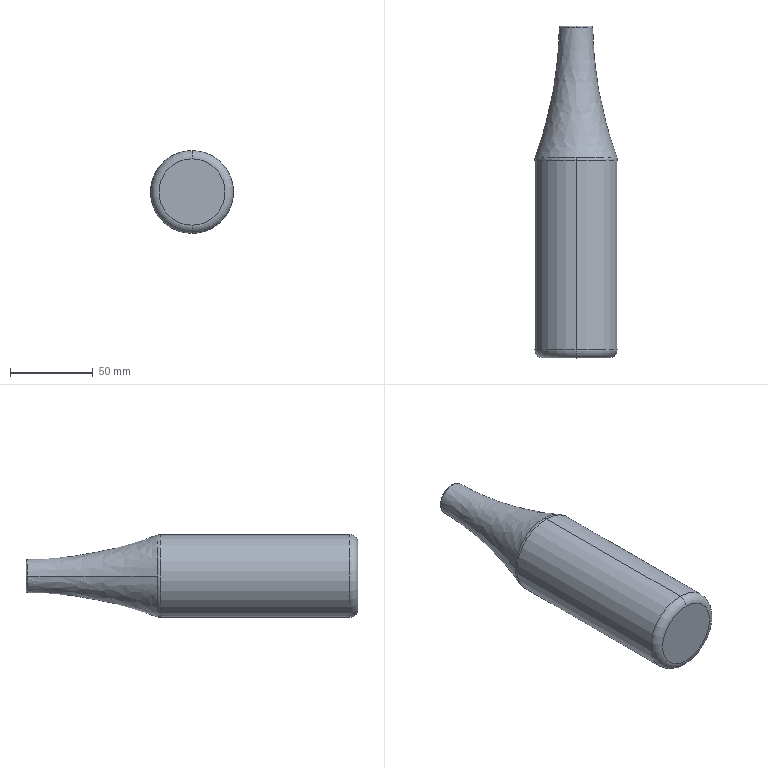Part | SolidWorks | features Fillet 2, Revolution 1, Shell 1 | 1 solid | 21 faces | box 50 x 200 x 50 mm | volume 77937 mm3 | torus 10 | spline 4 | cylinder 4 | plane 3 | commonest cylinder face diameters 44 x2 50 x2
STEP:
#1=CARTESIAN_POINT('',(-93.039,134.747,-7.013));
#2=VERTEX_POINT('',#1);
#3=CARTESIAN_POINT('',(-93.039,134.732,-7.013));
#4=VERTEX_POINT('',#3);
#5=CARTESIAN_POINT('',(-93.039,134.747,-8.013));
#6=DIRECTION('',(1.,0.,0.));
#7=DIRECTION('',(0.,0.,-1.));
#8=AXIS2_PLACEMENT_3D('',#5,#6,#7);
#9=CIRCLE('',#8,1.);
#10=EDGE_CURVE('',#2,#4,#9,.T.);
#11=ORIENTED_EDGE('',*,*,#10,.F.);
#12=CARTESIAN_POINT('',(-93.039,134.747,7.013));
#13=VERTEX_POINT('',#12);
#14=CARTESIAN_POINT('',(-93.039,134.747,0.));
#15=DIRECTION('',(0.,1.,0.));
#16=DIRECTION('',(0.,0.,1.));
#17=AXIS2_PLACEMENT_3D('',#14,#15,#16);
#18=CIRCLE('',#17,7.013);
#19=EDGE_CURVE('',#2,#13,#18,.T.);
#20=ORIENTED_EDGE('',*,*,#19,.T.);
#21=CARTESIAN_POINT('',(-93.039,134.732,7.013));
#22=VERTEX_POINT('',#21);
#23=CARTESIAN_POINT('',(-93.039,134.747,8.013));
#24=DIRECTION('',(-1.,0.,0.));
#25=DIRECTION('',(0.,0.,1.));
#26=AXIS2_PLACEMENT_3D('',#23,#24,#25);
#27=CIRCLE('',#26,1.);
#28=EDGE_CURVE('',#13,#22,#27,.T.);
#29=ORIENTED_EDGE('',*,*,#28,.T.);
#30=CARTESIAN_POINT('',(-100.052,134.732,0.));
#31=VERTEX_POINT('',#30);
#32=CARTESIAN_POINT('',(-93.039,134.732,0.));
#33=DIRECTION('',(0.,1.,0.));
#34=DIRECTION('',(0.,0.,1.));
#35=AXIS2_PLACEMENT_3D('',#32,#33,#34);
#36=CIRCLE('',#35,7.013);
#37=EDGE_CURVE('',#31,#22,#36,.T.);
#38=ORIENTED_EDGE('',*,*,#37,.F.);
#39=CARTESIAN_POINT('',(-93.039,134.732,0.));
#40=DIRECTION('',(0.,1.,0.));
#41=DIRECTION('',(0.,0.,1.));
#42=AXIS2_PLACEMENT_3D('',#39,#40,#41);
#43=CIRCLE('',#42,7.013);
#44=EDGE_CURVE('',#4,#31,#43,.T.);
#45=ORIENTED_EDGE('',*,*,#44,.F.);
#46=EDGE_LOOP('',(#11,#20,#29,#38,#45));
#47=FACE_OUTER_BOUND('',#46,.T.);
#48=CARTESIAN_POINT('',(-93.039,134.747,0.));
#49=DIRECTION('',(0.,1.,0.));
#50=DIRECTION('',(0.,0.,1.));
#51=AXIS2_PLACEMENT_3D('',#48,#49,#50);
#52=TOROIDAL_SURFACE('',#51,8.013,1.);
#53=ADVANCED_FACE('',(#47),#52,.T.);
#54=CARTESIAN_POINT('',(-86.026,134.732,0.));
#55=VERTEX_POINT('',#54);
#56=CARTESIAN_POINT('',(-93.039,134.732,0.));
#57=DIRECTION('',(0.,1.,0.));
#58=DIRECTION('',(0.,0.,1.));
#59=AXIS2_PLACEMENT_3D('',#56,#57,#58);
#60=CIRCLE('',#59,7.013);
#61=EDGE_CURVE('',#22,#55,#60,.T.);
#62=ORIENTED_EDGE('',*,*,#61,.T.);
#63=CARTESIAN_POINT('',(-71.039,55.211,0.));
#64=VERTEX_POINT('',#63);
#65=CARTESIAN_POINT('',(-86.026,134.732,0.));
#66=CARTESIAN_POINT('',(-85.624,107.792,0.));
#67=CARTESIAN_POINT('',(-80.621,81.268,0.));
#68=CARTESIAN_POINT('',(-71.039,55.211,0.));
#69=B_SPLINE_CURVE_WITH_KNOTS('',3,(#65,#66,#67,#68),.UNSPECIFIED.,.F.,.F.,(4,4),(0.01123,0.9355),.UNSPECIFIED.);
#70=EDGE_CURVE('',#55,#64,#69,.T.);
#71=ORIENTED_EDGE('',*,*,#70,.T.);
#72=CARTESIAN_POINT('',(-93.039,55.211,22.));
#73=VERTEX_POINT('',#72);
#74=CARTESIAN_POINT('',(-93.039,55.211,0.));
#75=DIRECTION('',(0.,1.,0.));
#76=DIRECTION('',(0.,0.,1.));
#77=AXIS2_PLACEMENT_3D('',#74,#75,#76);
#78=CIRCLE('',#77,22.);
#79=EDGE_CURVE('',#73,#64,#78,.T.);
#80=ORIENTED_EDGE('',*,*,#79,.F.);
#81=CARTESIAN_POINT('',(-115.039,55.211,0.));
#82=VERTEX_POINT('',#81);
#83=CARTESIAN_POINT('',(-93.039,55.211,0.));
#84=DIRECTION('',(0.,1.,0.));
#85=DIRECTION('',(0.,0.,1.));
#86=AXIS2_PLACEMENT_3D('',#83,#84,#85);
#87=CIRCLE('',#86,22.);
#88=EDGE_CURVE('',#82,#73,#87,.T.);
#89=ORIENTED_EDGE('',*,*,#88,.F.);
#90=CARTESIAN_POINT('',(-100.052,134.732,0.));
#91=CARTESIAN_POINT('',(-100.455,107.792,0.));
#92=CARTESIAN_POINT('',(-105.457,81.268,0.));
#93=CARTESIAN_POINT('',(-115.039,55.211,0.));
#94=B_SPLINE_CURVE_WITH_KNOTS('',3,(#90,#91,#92,#93),.UNSPECIFIED.,.F.,.F.,(4,4),(0.01123,0.9355),.UNSPECIFIED.);
#95=EDGE_CURVE('',#31,#82,#94,.T.);
#96=ORIENTED_EDGE('',*,*,#95,.F.);
#97=ORIENTED_EDGE('',*,*,#37,.T.);
#98=EDGE_LOOP('',(#62,#71,#80,#89,#96,#97));
#99=FACE_OUTER_BOUND('',#98,.T.);
#100=CARTESIAN_POINT('',(-100.052,134.732,0.));
#101=CARTESIAN_POINT('',(-100.052,134.732,14.026));
#102=CARTESIAN_POINT('',(-86.026,134.732,14.026));
#103=CARTESIAN_POINT('',(-86.026,134.732,0.));
#104=CARTESIAN_POINT('',(-100.455,107.792,0.));
#105=CARTESIAN_POINT('',(-100.455,107.792,14.831));
#106=CARTESIAN_POINT('',(-85.624,107.792,14.831));
#107=CARTESIAN_POINT('',(-85.624,107.792,0.));
#108=CARTESIAN_POINT('',(-105.457,81.268,0.));
#109=CARTESIAN_POINT('',(-105.457,81.268,24.836));
#110=CARTESIAN_POINT('',(-80.621,81.268,24.836));
#111=CARTESIAN_POINT('',(-80.621,81.268,0.));
#112=CARTESIAN_POINT('',(-115.039,55.211,0.));
#113=CARTESIAN_POINT('',(-115.039,55.211,44.));
#114=CARTESIAN_POINT('',(-71.039,55.211,44.));
#115=CARTESIAN_POINT('',(-71.039,55.211,0.));
#116=(BOUNDED_SURFACE()B_SPLINE_SURFACE(3,3,((#100,#101,#102,#103),(#104,#105,#106,#107),(#108,#109,#110,#111),(#112,#113,#114,#115)),.UNSPECIFIED.,.F.,.F.,.T.)B_SPLINE_SURFACE_WITH_KNOTS((4,4),(4,4),(0.,1.),(0.,1.),.UNSPECIFIED.)GEOMETRIC_REPRESENTATION_ITEM()RATIONAL_B_SPLINE_SURFACE(((1.,0.3333,0.3333,1.),(1.,0.3333,0.3333,1.),(1.,0.3333,0.3333,1.),(1.,0.3333,0.3333,1.)))REPRESENTATION_ITEM('')SURFACE());
#117=ADVANCED_FACE('',(#99),#116,.F.);
#118=CARTESIAN_POINT('',(-93.039,134.762,-10.013));
#119=VERTEX_POINT('',#118);
#120=CARTESIAN_POINT('',(-83.027,134.762,0.));
#121=VERTEX_POINT('',#120);
#122=CARTESIAN_POINT('',(-93.039,134.762,0.));
#123=DIRECTION('',(0.,-1.,0.));
#124=DIRECTION('',(0.,0.,1.));
#125=AXIS2_PLACEMENT_3D('',#122,#123,#124);
#126=CIRCLE('',#125,10.013);
#127=EDGE_CURVE('',#119,#121,#126,.T.);
#128=ORIENTED_EDGE('',*,*,#127,.T.);
#129=CARTESIAN_POINT('',(-68.344,56.575,0.));
#130=VERTEX_POINT('',#129);
#131=CARTESIAN_POINT('',(-83.027,134.762,0.));
#132=CARTESIAN_POINT('',(-82.431,95.042,0.));
#133=CARTESIAN_POINT('',(-68.344,56.575,0.));
#134=B_SPLINE_CURVE_WITH_KNOTS('',2,(#131,#132,#133),.UNSPECIFIED.,.F.,.F.,(3,3),(0.01141,0.9316),.UNSPECIFIED.);
#135=EDGE_CURVE('',#121,#130,#134,.T.);
#136=ORIENTED_EDGE('',*,*,#135,.T.);
#137=CARTESIAN_POINT('',(-93.039,56.575,-24.695));
#138=VERTEX_POINT('',#137);
#139=CARTESIAN_POINT('',(-93.039,56.575,0.));
#140=DIRECTION('',(0.,1.,0.));
#141=DIRECTION('',(0.,0.,1.));
#142=AXIS2_PLACEMENT_3D('',#139,#140,#141);
#143=CIRCLE('',#142,24.695);
#144=EDGE_CURVE('',#130,#138,#143,.T.);
#145=ORIENTED_EDGE('',*,*,#144,.T.);
#146=CARTESIAN_POINT('',(-117.734,56.575,0.));
#147=VERTEX_POINT('',#146);
#148=CARTESIAN_POINT('',(-93.039,56.575,0.));
#149=DIRECTION('',(0.,1.,0.));
#150=DIRECTION('',(0.,0.,1.));
#151=AXIS2_PLACEMENT_3D('',#148,#149,#150);
#152=CIRCLE('',#151,24.695);
#153=EDGE_CURVE('',#138,#147,#152,.T.);
#154=ORIENTED_EDGE('',*,*,#153,.T.);
#155=CARTESIAN_POINT('',(-103.052,134.762,0.));
#156=VERTEX_POINT('',#155);
#157=CARTESIAN_POINT('',(-103.052,134.762,0.));
#158=CARTESIAN_POINT('',(-103.648,95.042,0.));
#159=CARTESIAN_POINT('',(-117.734,56.575,0.));
#160=B_SPLINE_CURVE_WITH_KNOTS('',2,(#157,#158,#159),.UNSPECIFIED.,.F.,.F.,(3,3),(0.01141,0.9316),.UNSPECIFIED.);
#161=EDGE_CURVE('',#156,#147,#160,.T.);
#162=ORIENTED_EDGE('',*,*,#161,.F.);
#163=CARTESIAN_POINT('',(-93.039,134.762,0.));
#164=DIRECTION('',(0.,-1.,0.));
#165=DIRECTION('',(0.,0.,1.));
#166=AXIS2_PLACEMENT_3D('',#163,#164,#165);
#167=CIRCLE('',#166,10.013);
#168=EDGE_CURVE('',#156,#119,#167,.T.);
#169=ORIENTED_EDGE('',*,*,#168,.T.);
#170=EDGE_LOOP('',(#128,#136,#145,#154,#162,#169));
#171=FACE_OUTER_BOUND('',#170,.T.);
#172=CARTESIAN_POINT('',(-83.027,134.762,0.));
#173=CARTESIAN_POINT('',(-83.027,134.762,-20.025));
#174=CARTESIAN_POINT('',(-103.052,134.762,-20.025));
#175=CARTESIAN_POINT('',(-103.052,134.762,0.));
#176=CARTESIAN_POINT('',(-82.431,95.042,0.));
#177=CARTESIAN_POINT('',(-82.431,95.042,-21.217));
#178=CARTESIAN_POINT('',(-103.648,95.042,-21.217));
#179=CARTESIAN_POINT('',(-103.648,95.042,0.));
#180=CARTESIAN_POINT('',(-68.344,56.575,0.));
#181=CARTESIAN_POINT('',(-68.344,56.575,-49.39));
#182=CARTESIAN_POINT('',(-117.734,56.575,-49.39));
#183=CARTESIAN_POINT('',(-117.734,56.575,0.));
#184=(BOUNDED_SURFACE()B_SPLINE_SURFACE(2,3,((#172,#173,#174,#175),(#176,#177,#178,#179),(#180,#181,#182,#183)),.UNSPECIFIED.,.F.,.F.,.F.)B_SPLINE_SURFACE_WITH_KNOTS((3,3),(4,4),(0.01141,0.9316),(0.,1.),.UNSPECIFIED.)GEOMETRIC_REPRESENTATION_ITEM()RATIONAL_B_SPLINE_SURFACE(((1.,0.3333,0.3333,1.),(1.,0.3333,0.3333,1.),(1.,0.3333,0.3333,1.)))REPRESENTATION_ITEM('')SURFACE());
#185=ADVANCED_FACE('',(#171),#184,.T.);
#186=ORIENTED_EDGE('',*,*,#28,.F.);
#187=CARTESIAN_POINT('',(-93.039,134.747,0.));
#188=DIRECTION('',(0.,1.,0.));
#189=DIRECTION('',(0.,0.,1.));
#190=AXIS2_PLACEMENT_3D('',#187,#188,#189);
#191=CIRCLE('',#190,7.013);
#192=EDGE_CURVE('',#13,#2,#191,.T.);
#193=ORIENTED_EDGE('',*,*,#192,.T.);
#194=ORIENTED_EDGE('',*,*,#10,.T.);
#195=CARTESIAN_POINT('',(-93.039,134.732,0.));
#196=DIRECTION('',(0.,1.,0.));
#197=DIRECTION('',(0.,0.,1.));
#198=AXIS2_PLACEMENT_3D('',#195,#196,#197);
#199=CIRCLE('',#198,7.013);
#200=EDGE_CURVE('',#55,#4,#199,.T.);
#201=ORIENTED_EDGE('',*,*,#200,.F.);
#202=ORIENTED_EDGE('',*,*,#61,.F.);
#203=EDGE_LOOP('',(#186,#193,#194,#201,#202));
#204=FACE_OUTER_BOUND('',#203,.T.);
#205=CARTESIAN_POINT('',(-93.039,134.747,0.));
#206=DIRECTION('',(0.,1.,0.));
#207=DIRECTION('',(0.,0.,1.));
#208=AXIS2_PLACEMENT_3D('',#205,#206,#207);
#209=TOROIDAL_SURFACE('',#208,8.013,1.);
#210=ADVANCED_FACE('',(#204),#209,.T.);
#211=ORIENTED_EDGE('',*,*,#192,.F.);
#212=CARTESIAN_POINT('',(-93.039,135.747,8.013));
#213=VERTEX_POINT('',#212);
#214=CARTESIAN_POINT('',(-93.039,134.747,8.013));
#215=DIRECTION('',(-1.,0.,0.));
#216=DIRECTION('',(0.,0.,1.));
#217=AXIS2_PLACEMENT_3D('',#214,#215,#216);
#218=CIRCLE('',#217,1.);
#219=EDGE_CURVE('',#213,#13,#218,.T.);
#220=ORIENTED_EDGE('',*,*,#219,.F.);
#221=CARTESIAN_POINT('',(-93.039,135.747,-8.013));
#222=VERTEX_POINT('',#221);
#223=CARTESIAN_POINT('',(-93.039,135.747,0.));
#224=DIRECTION('',(0.,-1.,0.));
#225=DIRECTION('',(0.,0.,1.));
#226=AXIS2_PLACEMENT_3D('',#223,#224,#225);
#227=CIRCLE('',#226,8.013);
#228=EDGE_CURVE('',#222,#213,#227,.T.);
#229=ORIENTED_EDGE('',*,*,#228,.F.);
#230=CARTESIAN_POINT('',(-93.039,134.747,-8.013));
#231=DIRECTION('',(1.,0.,0.));
#232=DIRECTION('',(0.,0.,-1.));
#233=AXIS2_PLACEMENT_3D('',#230,#231,#232);
#234=CIRCLE('',#233,1.);
#235=EDGE_CURVE('',#222,#2,#234,.T.);
#236=ORIENTED_EDGE('',*,*,#235,.T.);
#237=EDGE_LOOP('',(#211,#220,#229,#236));
#238=FACE_OUTER_BOUND('',#237,.T.);
#239=CARTESIAN_POINT('',(-93.039,134.747,0.));
#240=DIRECTION('',(0.,1.,0.));
#241=DIRECTION('',(0.,0.,1.));
#242=AXIS2_PLACEMENT_3D('',#239,#240,#241);
#243=TOROIDAL_SURFACE('',#242,8.013,1.);
#244=ADVANCED_FACE('',(#238),#243,.T.);
#245=ORIENTED_EDGE('',*,*,#127,.F.);
#246=CARTESIAN_POINT('',(-93.039,135.747,-9.013));
#247=VERTEX_POINT('',#246);
#248=CARTESIAN_POINT('',(-93.039,134.747,-9.013));
#249=DIRECTION('',(1.,0.,0.));
#250=DIRECTION('',(0.,0.,-1.));
#251=AXIS2_PLACEMENT_3D('',#248,#249,#250);
#252=CIRCLE('',#251,1.);
#253=EDGE_CURVE('',#119,#247,#252,.T.);
#254=ORIENTED_EDGE('',*,*,#253,.T.);
#255=CARTESIAN_POINT('',(-93.039,135.747,9.013));
#256=VERTEX_POINT('',#255);
#257=CARTESIAN_POINT('',(-93.039,135.747,0.));
#258=DIRECTION('',(0.,1.,0.));
#259=DIRECTION('',(0.,0.,1.));
#260=AXIS2_PLACEMENT_3D('',#257,#258,#259);
#261=CIRCLE('',#260,9.013);
#262=EDGE_CURVE('',#256,#247,#261,.T.);
#263=ORIENTED_EDGE('',*,*,#262,.F.);
#264=CARTESIAN_POINT('',(-93.039,134.762,10.013));
#265=VERTEX_POINT('',#264);
#266=CARTESIAN_POINT('',(-93.039,134.747,9.013));
#267=DIRECTION('',(-1.,0.,0.));
#268=DIRECTION('',(0.,0.,1.));
#269=AXIS2_PLACEMENT_3D('',#266,#267,#268);
#270=CIRCLE('',#269,1.);
#271=EDGE_CURVE('',#265,#256,#270,.T.);
#272=ORIENTED_EDGE('',*,*,#271,.F.);
#273=CARTESIAN_POINT('',(-93.039,134.762,0.));
#274=DIRECTION('',(0.,-1.,0.));
#275=DIRECTION('',(0.,0.,1.));
#276=AXIS2_PLACEMENT_3D('',#273,#274,#275);
#277=CIRCLE('',#276,10.013);
#278=EDGE_CURVE('',#121,#265,#277,.T.);
#279=ORIENTED_EDGE('',*,*,#278,.F.);
#280=EDGE_LOOP('',(#245,#254,#263,#272,#279));
#281=FACE_OUTER_BOUND('',#280,.T.);
#282=CARTESIAN_POINT('',(-93.039,134.747,0.));
#283=DIRECTION('',(0.,1.,0.));
#284=DIRECTION('',(0.,0.,1.));
#285=AXIS2_PLACEMENT_3D('',#282,#283,#284);
#286=TOROIDAL_SURFACE('',#285,9.013,1.);
#287=ADVANCED_FACE('',(#281),#286,.T.);
#288=CARTESIAN_POINT('',(-93.039,-59.253,25.));
#289=VERTEX_POINT('',#288);
#290=CARTESIAN_POINT('',(-93.039,-59.253,-25.));
#291=VERTEX_POINT('',#290);
#292=CARTESIAN_POINT('',(-93.039,-59.253,0.));
#293=DIRECTION('',(0.,1.,0.));
#294=DIRECTION('',(0.,0.,-1.));
#295=AXIS2_PLACEMENT_3D('',#292,#293,#294);
#296=CIRCLE('',#295,25.);
#297=EDGE_CURVE('',#289,#291,#296,.T.);
#298=ORIENTED_EDGE('',*,*,#297,.F.);
#299=CARTESIAN_POINT('',(-93.039,-64.253,20.));
#300=VERTEX_POINT('',#299);
#301=CARTESIAN_POINT('',(-93.039,-59.253,20.));
#302=DIRECTION('',(1.,0.,0.));
#303=DIRECTION('',(0.,0.,-1.));
#304=AXIS2_PLACEMENT_3D('',#301,#302,#303);
#305=CIRCLE('',#304,5.);
#306=EDGE_CURVE('',#289,#300,#305,.T.);
#307=ORIENTED_EDGE('',*,*,#306,.T.);
#308=CARTESIAN_POINT('',(-93.039,-64.253,-20.));
#309=VERTEX_POINT('',#308);
#310=CARTESIAN_POINT('',(-93.039,-64.253,0.));
#311=DIRECTION('',(0.,-1.,0.));
#312=DIRECTION('',(0.,0.,-1.));
#313=AXIS2_PLACEMENT_3D('',#310,#311,#312);
#314=CIRCLE('',#313,20.);
#315=EDGE_CURVE('',#309,#300,#314,.T.);
#316=ORIENTED_EDGE('',*,*,#315,.F.);
#317=CARTESIAN_POINT('',(-93.039,-59.253,-20.));
#318=DIRECTION('',(-1.,0.,0.));
#319=DIRECTION('',(0.,0.,1.));
#320=AXIS2_PLACEMENT_3D('',#317,#318,#319);
#321=CIRCLE('',#320,5.);
#322=EDGE_CURVE('',#291,#309,#321,.T.);
#323=ORIENTED_EDGE('',*,*,#322,.F.);
#324=EDGE_LOOP('',(#298,#307,#316,#323));
#325=FACE_OUTER_BOUND('',#324,.T.);
#326=CARTESIAN_POINT('',(-93.039,-59.253,0.));
#327=DIRECTION('',(0.,-1.,0.));
#328=DIRECTION('',(0.,0.,-1.));
#329=AXIS2_PLACEMENT_3D('',#326,#327,#328);
#330=TOROIDAL_SURFACE('',#329,20.,5.);
#331=ADVANCED_FACE('',(#325),#330,.T.);
#332=CARTESIAN_POINT('',(-93.039,56.575,24.695));
#333=VERTEX_POINT('',#332);
#334=CARTESIAN_POINT('',(-93.039,56.575,0.));
#335=DIRECTION('',(0.,1.,0.));
#336=DIRECTION('',(0.,0.,1.));
#337=AXIS2_PLACEMENT_3D('',#334,#335,#336);
#338=CIRCLE('',#337,24.695);
#339=EDGE_CURVE('',#333,#130,#338,.T.);
#340=ORIENTED_EDGE('',*,*,#339,.F.);
#341=CARTESIAN_POINT('',(-93.039,54.856,25.));
#342=VERTEX_POINT('',#341);
#343=CARTESIAN_POINT('',(-93.039,54.856,20.));
#344=DIRECTION('',(1.,0.,0.));
#345=DIRECTION('',(0.,0.,-1.));
#346=AXIS2_PLACEMENT_3D('',#343,#344,#345);
#347=CIRCLE('',#346,5.);
#348=EDGE_CURVE('',#333,#342,#347,.T.);
#349=ORIENTED_EDGE('',*,*,#348,.T.);
#350=CARTESIAN_POINT('',(-93.039,54.856,-25.));
#351=VERTEX_POINT('',#350);
#352=CARTESIAN_POINT('',(-93.039,54.856,0.));
#353=DIRECTION('',(0.,-1.,0.));
#354=DIRECTION('',(0.,0.,-1.));
#355=AXIS2_PLACEMENT_3D('',#352,#353,#354);
#356=CIRCLE('',#355,25.);
#357=EDGE_CURVE('',#351,#342,#356,.T.);
#358=ORIENTED_EDGE('',*,*,#357,.F.);
#359=CARTESIAN_POINT('',(-93.039,54.856,-20.));
#360=DIRECTION('',(-1.,0.,0.));
#361=DIRECTION('',(0.,0.,1.));
#362=AXIS2_PLACEMENT_3D('',#359,#360,#361);
#363=CIRCLE('',#362,5.);
#364=EDGE_CURVE('',#138,#351,#363,.T.);
#365=ORIENTED_EDGE('',*,*,#364,.F.);
#366=ORIENTED_EDGE('',*,*,#144,.F.);
#367=EDGE_LOOP('',(#340,#349,#358,#365,#366));
#368=FACE_OUTER_BOUND('',#367,.T.);
#369=CARTESIAN_POINT('',(-93.039,54.856,0.));
#370=DIRECTION('',(0.,-1.,0.));
#371=DIRECTION('',(0.,0.,-1.));
#372=AXIS2_PLACEMENT_3D('',#369,#370,#371);
#373=TOROIDAL_SURFACE('',#372,20.,5.);
#374=ADVANCED_FACE('',(#368),#373,.T.);
#375=CARTESIAN_POINT('',(-93.039,-61.253,-22.));
#376=VERTEX_POINT('',#375);
#377=CARTESIAN_POINT('',(-93.039,-61.253,22.));
#378=VERTEX_POINT('',#377);
#379=CARTESIAN_POINT('',(-93.039,-61.253,0.));
#380=DIRECTION('',(0.,1.,0.));
#381=DIRECTION('',(0.,0.,-1.));
#382=AXIS2_PLACEMENT_3D('',#379,#380,#381);
#383=CIRCLE('',#382,22.);
#384=EDGE_CURVE('',#376,#378,#383,.T.);
#385=ORIENTED_EDGE('',*,*,#384,.F.);
#386=CARTESIAN_POINT('',(-93.039,55.211,-22.));
#387=VERTEX_POINT('',#386);
#388=CARTESIAN_POINT('',(-93.039,135.747,-22.));
#389=DIRECTION('',(0.,1.,0.));
#390=VECTOR('',#389,1000.);
#391=LINE('',#388,#390);
#392=EDGE_CURVE('',#376,#387,#391,.T.);
#393=ORIENTED_EDGE('',*,*,#392,.T.);
#394=CARTESIAN_POINT('',(-93.039,55.211,0.));
#395=DIRECTION('',(0.,1.,0.));
#396=DIRECTION('',(0.,0.,1.));
#397=AXIS2_PLACEMENT_3D('',#394,#395,#396);
#398=CIRCLE('',#397,22.);
#399=EDGE_CURVE('',#387,#82,#398,.T.);
#400=ORIENTED_EDGE('',*,*,#399,.T.);
#401=ORIENTED_EDGE('',*,*,#88,.T.);
#402=CARTESIAN_POINT('',(-93.039,135.747,22.));
#403=DIRECTION('',(0.,1.,0.));
#404=VECTOR('',#403,1000.);
#405=LINE('',#402,#404);
#406=EDGE_CURVE('',#378,#73,#405,.T.);
#407=ORIENTED_EDGE('',*,*,#406,.F.);
#408=EDGE_LOOP('',(#385,#393,#400,#401,#407));
#409=FACE_OUTER_BOUND('',#408,.T.);
#410=CARTESIAN_POINT('',(-93.039,135.747,0.));
#411=DIRECTION('',(0.,1.,0.));
#412=DIRECTION('',(0.,0.,1.));
#413=AXIS2_PLACEMENT_3D('',#410,#411,#412);
#414=CYLINDRICAL_SURFACE('',#413,22.);
#415=ADVANCED_FACE('',(#409),#414,.F.);
#416=ORIENTED_EDGE('',*,*,#297,.T.);
#417=CARTESIAN_POINT('',(-93.039,135.747,-25.));
#418=DIRECTION('',(0.,1.,0.));
#419=VECTOR('',#418,1000.);
#420=LINE('',#417,#419);
#421=EDGE_CURVE('',#291,#351,#420,.T.);
#422=ORIENTED_EDGE('',*,*,#421,.T.);
#423=ORIENTED_EDGE('',*,*,#357,.T.);
#424=CARTESIAN_POINT('',(-93.039,135.747,25.));
#425=DIRECTION('',(0.,1.,0.));
#426=VECTOR('',#425,1000.);
#427=LINE('',#424,#426);
#428=EDGE_CURVE('',#289,#342,#427,.T.);
#429=ORIENTED_EDGE('',*,*,#428,.F.);
#430=EDGE_LOOP('',(#416,#422,#423,#429));
#431=FACE_OUTER_BOUND('',#430,.T.);
#432=CARTESIAN_POINT('',(-93.039,135.747,0.));
#433=DIRECTION('',(0.,1.,0.));
#434=DIRECTION('',(0.,0.,1.));
#435=AXIS2_PLACEMENT_3D('',#432,#433,#434);
#436=CYLINDRICAL_SURFACE('',#435,25.);
#437=ADVANCED_FACE('',(#431),#436,.T.);
#438=ORIENTED_EDGE('',*,*,#262,.T.);
#439=CARTESIAN_POINT('',(-93.039,135.747,0.));
#440=DIRECTION('',(0.,1.,0.));
#441=DIRECTION('',(0.,0.,1.));
#442=AXIS2_PLACEMENT_3D('',#439,#440,#441);
#443=CIRCLE('',#442,9.013);
#444=EDGE_CURVE('',#247,#256,#443,.T.);
#445=ORIENTED_EDGE('',*,*,#444,.T.);
#446=EDGE_LOOP('',(#438,#445));
#447=FACE_OUTER_BOUND('',#446,.T.);
#448=CARTESIAN_POINT('',(-93.039,135.747,0.));
#449=DIRECTION('',(0.,-1.,0.));
#450=DIRECTION('',(0.,0.,1.));
#451=AXIS2_PLACEMENT_3D('',#448,#449,#450);
#452=CIRCLE('',#451,8.013);
#453=EDGE_CURVE('',#213,#222,#452,.T.);
#454=ORIENTED_EDGE('',*,*,#453,.T.);
#455=ORIENTED_EDGE('',*,*,#228,.T.);
#456=EDGE_LOOP('',(#454,#455));
#457=FACE_BOUND('',#456,.T.);
#458=CARTESIAN_POINT('',(-103.039,135.747,0.));
#459=DIRECTION('',(0.,1.,0.));
#460=DIRECTION('',(0.,0.,1.));
#461=AXIS2_PLACEMENT_3D('',#458,#459,#460);
#462=PLANE('',#461);
#463=ADVANCED_FACE('',(#447,#457),#462,.T.);
#464=ORIENTED_EDGE('',*,*,#315,.T.);
#465=CARTESIAN_POINT('',(-93.039,-64.253,0.));
#466=DIRECTION('',(0.,-1.,0.));
#467=DIRECTION('',(0.,0.,-1.));
#468=AXIS2_PLACEMENT_3D('',#465,#466,#467);
#469=CIRCLE('',#468,20.);
#470=EDGE_CURVE('',#300,#309,#469,.T.);
#471=ORIENTED_EDGE('',*,*,#470,.T.);
#472=EDGE_LOOP('',(#464,#471));
#473=FACE_OUTER_BOUND('',#472,.T.);
#474=CARTESIAN_POINT('',(-118.039,-64.253,0.));
#475=DIRECTION('',(0.,-1.,0.));
#476=DIRECTION('',(0.,0.,-1.));
#477=AXIS2_PLACEMENT_3D('',#474,#475,#476);
#478=PLANE('',#477);
#479=ADVANCED_FACE('',(#473),#478,.T.);
#480=ORIENTED_EDGE('',*,*,#421,.F.);
#481=CARTESIAN_POINT('',(-93.039,-59.253,0.));
#482=DIRECTION('',(0.,1.,0.));
#483=DIRECTION('',(0.,0.,-1.));
#484=AXIS2_PLACEMENT_3D('',#481,#482,#483);
#485=CIRCLE('',#484,25.);
#486=EDGE_CURVE('',#291,#289,#485,.T.);
#487=ORIENTED_EDGE('',*,*,#486,.T.);
#488=ORIENTED_EDGE('',*,*,#428,.T.);
#489=CARTESIAN_POINT('',(-93.039,54.856,0.));
#490=DIRECTION('',(0.,-1.,0.));
#491=DIRECTION('',(0.,0.,-1.));
#492=AXIS2_PLACEMENT_3D('',#489,#490,#491);
#493=CIRCLE('',#492,25.);
#494=EDGE_CURVE('',#342,#351,#493,.T.);
#495=ORIENTED_EDGE('',*,*,#494,.T.);
#496=EDGE_LOOP('',(#480,#487,#488,#495));
#497=FACE_OUTER_BOUND('',#496,.T.);
#498=CARTESIAN_POINT('',(-93.039,135.747,0.));
#499=DIRECTION('',(0.,1.,0.));
#500=DIRECTION('',(0.,0.,1.));
#501=AXIS2_PLACEMENT_3D('',#498,#499,#500);
#502=CYLINDRICAL_SURFACE('',#501,25.);
#503=ADVANCED_FACE('',(#497),#502,.T.);
#504=ORIENTED_EDGE('',*,*,#135,.F.);
#505=ORIENTED_EDGE('',*,*,#278,.T.);
#506=CARTESIAN_POINT('',(-93.039,134.762,0.));
#507=DIRECTION('',(0.,-1.,0.));
#508=DIRECTION('',(0.,0.,1.));
#509=AXIS2_PLACEMENT_3D('',#506,#507,#508);
#510=CIRCLE('',#509,10.013);
#511=EDGE_CURVE('',#265,#156,#510,.T.);
#512=ORIENTED_EDGE('',*,*,#511,.T.);
#513=ORIENTED_EDGE('',*,*,#161,.T.);
#514=CARTESIAN_POINT('',(-93.039,56.575,0.));
#515=DIRECTION('',(0.,1.,0.));
#516=DIRECTION('',(0.,0.,1.));
#517=AXIS2_PLACEMENT_3D('',#514,#515,#516);
#518=CIRCLE('',#517,24.695);
#519=EDGE_CURVE('',#147,#333,#518,.T.);
#520=ORIENTED_EDGE('',*,*,#519,.T.);
#521=ORIENTED_EDGE('',*,*,#339,.T.);
#522=EDGE_LOOP('',(#504,#505,#512,#513,#520,#521));
#523=FACE_OUTER_BOUND('',#522,.T.);
#524=CARTESIAN_POINT('',(-103.052,134.762,0.));
#525=CARTESIAN_POINT('',(-103.052,134.762,20.025));
#526=CARTESIAN_POINT('',(-83.027,134.762,20.025));
#527=CARTESIAN_POINT('',(-83.027,134.762,0.));
#528=CARTESIAN_POINT('',(-103.648,95.042,0.));
#529=CARTESIAN_POINT('',(-103.648,95.042,21.217));
#530=CARTESIAN_POINT('',(-82.431,95.042,21.217));
#531=CARTESIAN_POINT('',(-82.431,95.042,0.));
#532=CARTESIAN_POINT('',(-117.734,56.575,0.));
#533=CARTESIAN_POINT('',(-117.734,56.575,49.39));
#534=CARTESIAN_POINT('',(-68.344,56.575,49.39));
#535=CARTESIAN_POINT('',(-68.344,56.575,0.));
#536=(BOUNDED_SURFACE()B_SPLINE_SURFACE(2,3,((#524,#525,#526,#527),(#528,#529,#530,#531),(#532,#533,#534,#535)),.UNSPECIFIED.,.F.,.F.,.T.)B_SPLINE_SURFACE_WITH_KNOTS((3,3),(4,4),(0.01141,0.9316),(0.,1.),.UNSPECIFIED.)GEOMETRIC_REPRESENTATION_ITEM()RATIONAL_B_SPLINE_SURFACE(((1.,0.3333,0.3333,1.),(1.,0.3333,0.3333,1.),(1.,0.3333,0.3333,1.)))REPRESENTATION_ITEM('')SURFACE());
#537=ADVANCED_FACE('',(#523),#536,.T.);
#538=CARTESIAN_POINT('',(-93.039,-61.253,0.));
#539=DIRECTION('',(0.,1.,0.));
#540=DIRECTION('',(0.,0.,-1.));
#541=AXIS2_PLACEMENT_3D('',#538,#539,#540);
#542=CIRCLE('',#541,22.);
#543=EDGE_CURVE('',#378,#376,#542,.T.);
#544=ORIENTED_EDGE('',*,*,#543,.T.);
#545=ORIENTED_EDGE('',*,*,#384,.T.);
#546=EDGE_LOOP('',(#544,#545));
#547=FACE_OUTER_BOUND('',#546,.T.);
#548=CARTESIAN_POINT('',(-118.039,-61.253,0.));
#549=DIRECTION('',(0.,-1.,0.));
#550=DIRECTION('',(0.,0.,-1.));
#551=AXIS2_PLACEMENT_3D('',#548,#549,#550);
#552=PLANE('',#551);
#553=ADVANCED_FACE('',(#547),#552,.F.);
#554=ORIENTED_EDGE('',*,*,#392,.F.);
#555=ORIENTED_EDGE('',*,*,#543,.F.);
#556=ORIENTED_EDGE('',*,*,#406,.T.);
#557=ORIENTED_EDGE('',*,*,#79,.T.);
#558=CARTESIAN_POINT('',(-93.039,55.211,0.));
#559=DIRECTION('',(0.,1.,0.));
#560=DIRECTION('',(0.,0.,1.));
#561=AXIS2_PLACEMENT_3D('',#558,#559,#560);
#562=CIRCLE('',#561,22.);
#563=EDGE_CURVE('',#64,#387,#562,.T.);
#564=ORIENTED_EDGE('',*,*,#563,.T.);
#565=EDGE_LOOP('',(#554,#555,#556,#557,#564));
#566=FACE_OUTER_BOUND('',#565,.T.);
#567=CARTESIAN_POINT('',(-93.039,135.747,0.));
#568=DIRECTION('',(0.,1.,0.));
#569=DIRECTION('',(0.,0.,1.));
#570=AXIS2_PLACEMENT_3D('',#567,#568,#569);
#571=CYLINDRICAL_SURFACE('',#570,22.);
#572=ADVANCED_FACE('',(#566),#571,.F.);
#573=ORIENTED_EDGE('',*,*,#70,.F.);
#574=ORIENTED_EDGE('',*,*,#200,.T.);
#575=ORIENTED_EDGE('',*,*,#44,.T.);
#576=ORIENTED_EDGE('',*,*,#95,.T.);
#577=ORIENTED_EDGE('',*,*,#399,.F.);
#578=ORIENTED_EDGE('',*,*,#563,.F.);
#579=EDGE_LOOP('',(#573,#574,#575,#576,#577,#578));
#580=FACE_OUTER_BOUND('',#579,.T.);
#581=CARTESIAN_POINT('',(-86.026,134.732,0.));
#582=CARTESIAN_POINT('',(-86.026,134.732,-14.026));
#583=CARTESIAN_POINT('',(-100.052,134.732,-14.026));
#584=CARTESIAN_POINT('',(-100.052,134.732,0.));
#585=CARTESIAN_POINT('',(-85.624,107.792,0.));
#586=CARTESIAN_POINT('',(-85.624,107.792,-14.831));
#587=CARTESIAN_POINT('',(-100.455,107.792,-14.831));
#588=CARTESIAN_POINT('',(-100.455,107.792,0.));
#589=CARTESIAN_POINT('',(-80.621,81.268,0.));
#590=CARTESIAN_POINT('',(-80.621,81.268,-24.836));
#591=CARTESIAN_POINT('',(-105.457,81.268,-24.836));
#592=CARTESIAN_POINT('',(-105.457,81.268,0.));
#593=CARTESIAN_POINT('',(-71.039,55.211,0.));
#594=CARTESIAN_POINT('',(-71.039,55.211,-44.));
#595=CARTESIAN_POINT('',(-115.039,55.211,-44.));
#596=CARTESIAN_POINT('',(-115.039,55.211,0.));
#597=(BOUNDED_SURFACE()B_SPLINE_SURFACE(3,3,((#581,#582,#583,#584),(#585,#586,#587,#588),(#589,#590,#591,#592),(#593,#594,#595,#596)),.UNSPECIFIED.,.F.,.F.,.T.)B_SPLINE_SURFACE_WITH_KNOTS((4,4),(4,4),(0.,1.),(0.,1.),.UNSPECIFIED.)GEOMETRIC_REPRESENTATION_ITEM()RATIONAL_B_SPLINE_SURFACE(((1.,0.3333,0.3333,1.),(1.,0.3333,0.3333,1.),(1.,0.3333,0.3333,1.),(1.,0.3333,0.3333,1.)))REPRESENTATION_ITEM('')SURFACE());
#598=ADVANCED_FACE('',(#580),#597,.F.);
#599=ORIENTED_EDGE('',*,*,#348,.F.);
#600=ORIENTED_EDGE('',*,*,#519,.F.);
#601=ORIENTED_EDGE('',*,*,#153,.F.);
#602=ORIENTED_EDGE('',*,*,#364,.T.);
#603=ORIENTED_EDGE('',*,*,#494,.F.);
#604=EDGE_LOOP('',(#599,#600,#601,#602,#603));
#605=FACE_OUTER_BOUND('',#604,.T.);
#606=CARTESIAN_POINT('',(-93.039,54.856,0.));
#607=DIRECTION('',(0.,-1.,0.));
#608=DIRECTION('',(0.,0.,-1.));
#609=AXIS2_PLACEMENT_3D('',#606,#607,#608);
#610=TOROIDAL_SURFACE('',#609,20.,5.);
#611=ADVANCED_FACE('',(#605),#610,.T.);
#612=ORIENTED_EDGE('',*,*,#306,.F.);
#613=ORIENTED_EDGE('',*,*,#486,.F.);
#614=ORIENTED_EDGE('',*,*,#322,.T.);
#615=ORIENTED_EDGE('',*,*,#470,.F.);
#616=EDGE_LOOP('',(#612,#613,#614,#615));
#617=FACE_OUTER_BOUND('',#616,.T.);
#618=CARTESIAN_POINT('',(-93.039,-59.253,0.));
#619=DIRECTION('',(0.,-1.,0.));
#620=DIRECTION('',(0.,0.,-1.));
#621=AXIS2_PLACEMENT_3D('',#618,#619,#620);
#622=TOROIDAL_SURFACE('',#621,20.,5.);
#623=ADVANCED_FACE('',(#617),#622,.T.);
#624=ORIENTED_EDGE('',*,*,#253,.F.);
#625=ORIENTED_EDGE('',*,*,#168,.F.);
#626=ORIENTED_EDGE('',*,*,#511,.F.);
#627=ORIENTED_EDGE('',*,*,#271,.T.);
#628=ORIENTED_EDGE('',*,*,#444,.F.);
#629=EDGE_LOOP('',(#624,#625,#626,#627,#628));
#630=FACE_OUTER_BOUND('',#629,.T.);
#631=CARTESIAN_POINT('',(-93.039,134.747,0.));
#632=DIRECTION('',(0.,1.,0.));
#633=DIRECTION('',(0.,0.,1.));
#634=AXIS2_PLACEMENT_3D('',#631,#632,#633);
#635=TOROIDAL_SURFACE('',#634,9.013,1.);
#636=ADVANCED_FACE('',(#630),#635,.T.);
#637=ORIENTED_EDGE('',*,*,#19,.F.);
#638=ORIENTED_EDGE('',*,*,#235,.F.);
#639=ORIENTED_EDGE('',*,*,#453,.F.);
#640=ORIENTED_EDGE('',*,*,#219,.T.);
#641=EDGE_LOOP('',(#637,#638,#639,#640));
#642=FACE_OUTER_BOUND('',#641,.T.);
#643=CARTESIAN_POINT('',(-93.039,134.747,0.));
#644=DIRECTION('',(0.,1.,0.));
#645=DIRECTION('',(0.,0.,1.));
#646=AXIS2_PLACEMENT_3D('',#643,#644,#645);
#647=TOROIDAL_SURFACE('',#646,8.013,1.);
#648=ADVANCED_FACE('',(#642),#647,.T.);
#649=CLOSED_SHELL('',(#53,#117,#185,#210,#244,#287,#331,#374,#415,#437,#463,#479,#503,#537,#553,#572,#598,#611,#623,#636,#648));
#650=MANIFOLD_SOLID_BREP('',#649);
#651=CARTESIAN_POINT('',(0.,0.,0.));
#652=DIRECTION('',(0.,0.,1.));
#653=DIRECTION('',(1.,0.,0.));
#654=AXIS2_PLACEMENT_3D('',#651,#652,#653);
#655=(LENGTH_UNIT()NAMED_UNIT(*)SI_UNIT(.MILLI.,.METRE.));
#656=UNCERTAINTY_MEASURE_WITH_UNIT(LENGTH_MEASURE(0.00001),#655,'','');
#657=(NAMED_UNIT(*)PLANE_ANGLE_UNIT()SI_UNIT($,.RADIAN.));
#658=(NAMED_UNIT(*)SI_UNIT($,.STERADIAN.)SOLID_ANGLE_UNIT());
#659=(GEOMETRIC_REPRESENTATION_CONTEXT(3)GLOBAL_UNCERTAINTY_ASSIGNED_CONTEXT((#656))GLOBAL_UNIT_ASSIGNED_CONTEXT((#655,#657,#658))REPRESENTATION_CONTEXT('',''));
#660=ADVANCED_BREP_SHAPE_REPRESENTATION('',(#650,#654),#659);